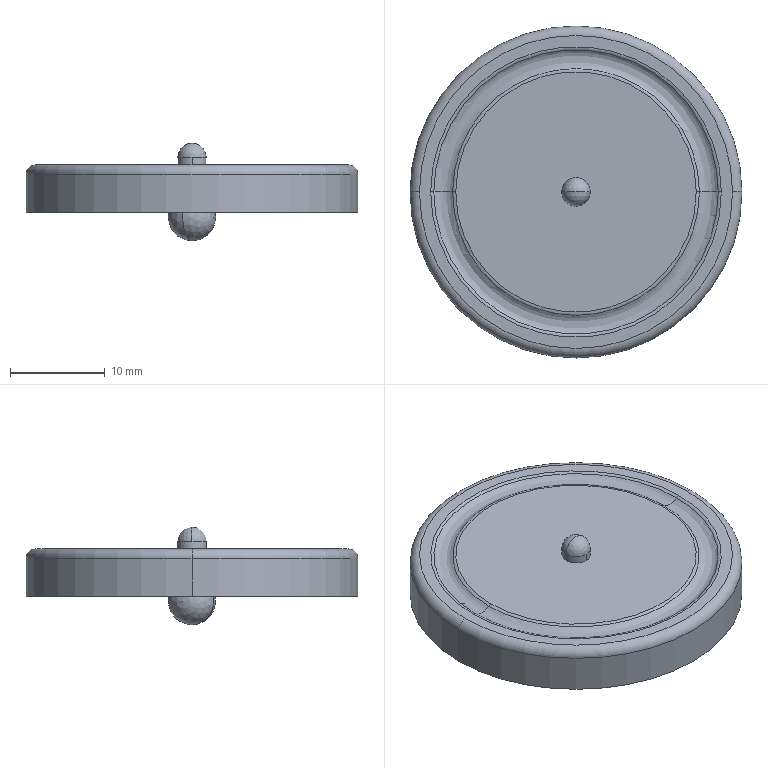Part | SolidWorks | features Fillet 2, RevCut 2, Revolution 2, Extrusion 1 | 2 solids | 24 faces | box 35 x 35 x 10.3 mm | volume 4614 mm3 | torus 10 | cylinder 6 | sphere 4 | plane 4 | commonest cylinder face diameters 3 x2 11 x2 35 x2
STEP:
#1=CARTESIAN_POINT('',(-121.531,115.619,-3.));
#2=VERTEX_POINT('',#1);
#3=CARTESIAN_POINT('',(-121.531,115.619,2.));
#4=VERTEX_POINT('',#3);
#5=CARTESIAN_POINT('',(-121.531,115.619,-0.5));
#6=DIRECTION('',(0.9209,-0.3898,0.));
#7=DIRECTION('',(0.3898,0.9209,0.));
#8=AXIS2_PLACEMENT_3D('',#5,#6,#7);
#9=CIRCLE('',#8,2.5);
#10=EDGE_CURVE('',#2,#4,#9,.T.);
#11=ORIENTED_EDGE('',*,*,#10,.F.);
#12=CARTESIAN_POINT('',(-121.531,115.619,-0.5));
#13=DIRECTION('',(-0.9209,0.3898,0.));
#14=DIRECTION('',(-0.3898,-0.9209,0.));
#15=AXIS2_PLACEMENT_3D('',#12,#13,#14);
#16=CIRCLE('',#15,2.5);
#17=EDGE_CURVE('',#2,#4,#16,.T.);
#18=ORIENTED_EDGE('',*,*,#17,.T.);
#19=EDGE_LOOP('',(#11,#18));
#20=FACE_OUTER_BOUND('',#19,.T.);
#21=CARTESIAN_POINT('',(-121.531,115.619,-0.5));
#22=DIRECTION('',(-0.9209,0.3898,0.));
#23=DIRECTION('',(0.3898,0.9209,0.));
#24=AXIS2_PLACEMENT_3D('',#21,#22,#23);
#25=SPHERICAL_SURFACE('',#24,2.5);
#26=ADVANCED_FACE('',(#20),#25,.T.);
#27=ORIENTED_EDGE('',*,*,#17,.F.);
#28=ORIENTED_EDGE('',*,*,#10,.T.);
#29=EDGE_LOOP('',(#27,#28));
#30=FACE_OUTER_BOUND('',#29,.T.);
#31=CARTESIAN_POINT('',(-121.531,115.619,-0.5));
#32=DIRECTION('',(-0.9209,0.3898,0.));
#33=DIRECTION('',(0.3898,0.9209,0.));
#34=AXIS2_PLACEMENT_3D('',#31,#32,#33);
#35=SPHERICAL_SURFACE('',#34,2.5);
#36=ADVANCED_FACE('',(#30),#35,.T.);
#37=CLOSED_SHELL('',(#26,#36));
#38=MANIFOLD_SOLID_BREP('',#37);
#39=CARTESIAN_POINT('',(-120.031,115.619,5.8));
#40=VERTEX_POINT('',#39);
#41=CARTESIAN_POINT('',(-121.531,114.119,5.8));
#42=VERTEX_POINT('',#41);
#43=CARTESIAN_POINT('',(-121.531,115.619,5.8));
#44=DIRECTION('',(0.,0.,-1.));
#45=DIRECTION('',(0.,1.,0.));
#46=AXIS2_PLACEMENT_3D('',#43,#44,#45);
#47=CIRCLE('',#46,1.5);
#48=EDGE_CURVE('',#40,#42,#47,.T.);
#49=ORIENTED_EDGE('',*,*,#48,.T.);
#50=CARTESIAN_POINT('',(-121.531,114.119,5.));
#51=VERTEX_POINT('',#50);
#52=CARTESIAN_POINT('',(-121.531,114.119,0.));
#53=DIRECTION('',(0.,0.,-1.));
#54=VECTOR('',#53,1000.);
#55=LINE('',#52,#54);
#56=EDGE_CURVE('',#42,#51,#55,.T.);
#57=ORIENTED_EDGE('',*,*,#56,.T.);
#58=CARTESIAN_POINT('',(-121.531,117.119,5.));
#59=VERTEX_POINT('',#58);
#60=CARTESIAN_POINT('',(-121.531,115.619,5.));
#61=DIRECTION('',(0.,0.,-1.));
#62=DIRECTION('',(1.,0.,0.));
#63=AXIS2_PLACEMENT_3D('',#60,#61,#62);
#64=CIRCLE('',#63,1.5);
#65=EDGE_CURVE('',#59,#51,#64,.T.);
#66=ORIENTED_EDGE('',*,*,#65,.F.);
#67=CARTESIAN_POINT('',(-121.531,117.119,5.8));
#68=VERTEX_POINT('',#67);
#69=CARTESIAN_POINT('',(-121.531,117.119,0.));
#70=DIRECTION('',(0.,0.,-1.));
#71=VECTOR('',#70,1000.);
#72=LINE('',#69,#71);
#73=EDGE_CURVE('',#68,#59,#72,.T.);
#74=ORIENTED_EDGE('',*,*,#73,.F.);
#75=CARTESIAN_POINT('',(-121.531,115.619,5.8));
#76=DIRECTION('',(0.,0.,-1.));
#77=DIRECTION('',(0.,1.,0.));
#78=AXIS2_PLACEMENT_3D('',#75,#76,#77);
#79=CIRCLE('',#78,1.5);
#80=EDGE_CURVE('',#68,#40,#79,.T.);
#81=ORIENTED_EDGE('',*,*,#80,.T.);
#82=EDGE_LOOP('',(#49,#57,#66,#74,#81));
#83=FACE_OUTER_BOUND('',#82,.T.);
#84=CARTESIAN_POINT('',(-121.531,115.619,0.));
#85=DIRECTION('',(0.,0.,-1.));
#86=DIRECTION('',(0.,1.,0.));
#87=AXIS2_PLACEMENT_3D('',#84,#85,#86);
#88=CYLINDRICAL_SURFACE('',#87,1.5);
#89=ADVANCED_FACE('',(#83),#88,.T.);
#90=CARTESIAN_POINT('',(-121.531,115.619,7.3));
#91=VERTEX_POINT('',#90);
#92=CARTESIAN_POINT('',(-121.531,115.619,5.8));
#93=DIRECTION('',(0.,1.,0.));
#94=DIRECTION('',(0.,0.,1.));
#95=AXIS2_PLACEMENT_3D('',#92,#93,#94);
#96=CIRCLE('',#95,1.5);
#97=EDGE_CURVE('',#91,#40,#96,.T.);
#98=ORIENTED_EDGE('',*,*,#97,.F.);
#99=CARTESIAN_POINT('',(-123.031,115.619,5.8));
#100=VERTEX_POINT('',#99);
#101=CARTESIAN_POINT('',(-121.531,115.619,5.8));
#102=DIRECTION('',(0.,-1.,0.));
#103=DIRECTION('',(0.,0.,-1.));
#104=AXIS2_PLACEMENT_3D('',#101,#102,#103);
#105=CIRCLE('',#104,1.5);
#106=EDGE_CURVE('',#91,#100,#105,.T.);
#107=ORIENTED_EDGE('',*,*,#106,.T.);
#108=CARTESIAN_POINT('',(-121.531,115.619,5.8));
#109=DIRECTION('',(0.,0.,-1.));
#110=DIRECTION('',(0.,1.,0.));
#111=AXIS2_PLACEMENT_3D('',#108,#109,#110);
#112=CIRCLE('',#111,1.5);
#113=EDGE_CURVE('',#42,#100,#112,.T.);
#114=ORIENTED_EDGE('',*,*,#113,.F.);
#115=ORIENTED_EDGE('',*,*,#48,.F.);
#116=EDGE_LOOP('',(#98,#107,#114,#115));
#117=FACE_OUTER_BOUND('',#116,.T.);
#118=CARTESIAN_POINT('',(-121.531,115.619,5.8));
#119=DIRECTION('',(0.,-1.,0.));
#120=DIRECTION('',(1.,0.,0.));
#121=AXIS2_PLACEMENT_3D('',#118,#119,#120);
#122=SPHERICAL_SURFACE('',#121,1.5);
#123=ADVANCED_FACE('',(#117),#122,.T.);
#124=CARTESIAN_POINT('',(-108.854,115.619,5.));
#125=VERTEX_POINT('',#124);
#126=CARTESIAN_POINT('',(-134.208,115.619,5.));
#127=VERTEX_POINT('',#126);
#128=CARTESIAN_POINT('',(-121.531,115.619,5.));
#129=DIRECTION('',(0.,0.,1.));
#130=DIRECTION('',(1.,0.,0.));
#131=AXIS2_PLACEMENT_3D('',#128,#129,#130);
#132=CIRCLE('',#131,12.677);
#133=EDGE_CURVE('',#125,#127,#132,.T.);
#134=ORIENTED_EDGE('',*,*,#133,.F.);
#135=CARTESIAN_POINT('',(-108.523,115.619,4.875));
#136=VERTEX_POINT('',#135);
#137=CARTESIAN_POINT('',(-108.854,115.619,4.5));
#138=DIRECTION('',(0.,1.,0.));
#139=DIRECTION('',(-1.,0.,0.));
#140=AXIS2_PLACEMENT_3D('',#137,#138,#139);
#141=CIRCLE('',#140,0.5);
#142=EDGE_CURVE('',#125,#136,#141,.T.);
#143=ORIENTED_EDGE('',*,*,#142,.T.);
#144=CARTESIAN_POINT('',(-134.539,115.619,4.875));
#145=VERTEX_POINT('',#144);
#146=CARTESIAN_POINT('',(-121.531,115.619,4.875));
#147=DIRECTION('',(0.,0.,-1.));
#148=DIRECTION('',(1.,0.,0.));
#149=AXIS2_PLACEMENT_3D('',#146,#147,#148);
#150=CIRCLE('',#149,13.008);
#151=EDGE_CURVE('',#145,#136,#150,.T.);
#152=ORIENTED_EDGE('',*,*,#151,.F.);
#153=CARTESIAN_POINT('',(-134.208,115.619,4.5));
#154=DIRECTION('',(0.,-1.,0.));
#155=DIRECTION('',(0.,0.,-1.));
#156=AXIS2_PLACEMENT_3D('',#153,#154,#155);
#157=CIRCLE('',#156,0.5);
#158=EDGE_CURVE('',#127,#145,#157,.T.);
#159=ORIENTED_EDGE('',*,*,#158,.F.);
#160=EDGE_LOOP('',(#134,#143,#152,#159));
#161=FACE_OUTER_BOUND('',#160,.T.);
#162=CARTESIAN_POINT('',(-121.531,115.619,4.5));
#163=DIRECTION('',(0.,0.,-1.));
#164=DIRECTION('',(-1.,0.,0.));
#165=AXIS2_PLACEMENT_3D('',#162,#163,#164);
#166=TOROIDAL_SURFACE('',#165,12.677,0.5);
#167=ADVANCED_FACE('',(#161),#166,.T.);
#168=CARTESIAN_POINT('',(-136.854,115.619,5.));
#169=VERTEX_POINT('',#168);
#170=CARTESIAN_POINT('',(-106.208,115.619,5.));
#171=VERTEX_POINT('',#170);
#172=CARTESIAN_POINT('',(-121.531,115.619,5.));
#173=DIRECTION('',(0.,0.,-1.));
#174=DIRECTION('',(1.,0.,0.));
#175=AXIS2_PLACEMENT_3D('',#172,#173,#174);
#176=CIRCLE('',#175,15.323);
#177=EDGE_CURVE('',#169,#171,#176,.T.);
#178=ORIENTED_EDGE('',*,*,#177,.F.);
#179=CARTESIAN_POINT('',(-136.523,115.619,4.875));
#180=VERTEX_POINT('',#179);
#181=CARTESIAN_POINT('',(-136.854,115.619,4.5));
#182=DIRECTION('',(0.,1.,0.));
#183=DIRECTION('',(-1.,0.,0.));
#184=AXIS2_PLACEMENT_3D('',#181,#182,#183);
#185=CIRCLE('',#184,0.5);
#186=EDGE_CURVE('',#169,#180,#185,.T.);
#187=ORIENTED_EDGE('',*,*,#186,.T.);
#188=CARTESIAN_POINT('',(-106.539,115.619,4.875));
#189=VERTEX_POINT('',#188);
#190=CARTESIAN_POINT('',(-121.531,115.619,4.875));
#191=DIRECTION('',(0.,0.,1.));
#192=DIRECTION('',(1.,0.,0.));
#193=AXIS2_PLACEMENT_3D('',#190,#191,#192);
#194=CIRCLE('',#193,14.992);
#195=EDGE_CURVE('',#189,#180,#194,.T.);
#196=ORIENTED_EDGE('',*,*,#195,.F.);
#197=CARTESIAN_POINT('',(-106.208,115.619,4.5));
#198=DIRECTION('',(0.,-1.,0.));
#199=DIRECTION('',(0.,0.,-1.));
#200=AXIS2_PLACEMENT_3D('',#197,#198,#199);
#201=CIRCLE('',#200,0.5);
#202=EDGE_CURVE('',#171,#189,#201,.T.);
#203=ORIENTED_EDGE('',*,*,#202,.F.);
#204=EDGE_LOOP('',(#178,#187,#196,#203));
#205=FACE_OUTER_BOUND('',#204,.T.);
#206=CARTESIAN_POINT('',(-121.531,115.619,4.5));
#207=DIRECTION('',(0.,0.,1.));
#208=DIRECTION('',(1.,0.,0.));
#209=AXIS2_PLACEMENT_3D('',#206,#207,#208);
#210=TOROIDAL_SURFACE('',#209,15.323,0.5);
#211=ADVANCED_FACE('',(#205),#210,.T.);
#212=CARTESIAN_POINT('',(-139.031,115.619,4.));
#213=VERTEX_POINT('',#212);
#214=CARTESIAN_POINT('',(-104.031,115.619,4.));
#215=VERTEX_POINT('',#214);
#216=CARTESIAN_POINT('',(-121.531,115.619,4.));
#217=DIRECTION('',(0.,0.,-1.));
#218=DIRECTION('',(1.,0.,0.));
#219=AXIS2_PLACEMENT_3D('',#216,#217,#218);
#220=CIRCLE('',#219,17.5);
#221=EDGE_CURVE('',#213,#215,#220,.T.);
#222=ORIENTED_EDGE('',*,*,#221,.F.);
#223=CARTESIAN_POINT('',(-138.031,115.619,5.));
#224=VERTEX_POINT('',#223);
#225=CARTESIAN_POINT('',(-138.031,115.619,4.));
#226=DIRECTION('',(0.,1.,0.));
#227=DIRECTION('',(-1.,0.,0.));
#228=AXIS2_PLACEMENT_3D('',#225,#226,#227);
#229=CIRCLE('',#228,1.);
#230=EDGE_CURVE('',#213,#224,#229,.T.);
#231=ORIENTED_EDGE('',*,*,#230,.T.);
#232=CARTESIAN_POINT('',(-105.031,115.619,5.));
#233=VERTEX_POINT('',#232);
#234=CARTESIAN_POINT('',(-121.531,115.619,5.));
#235=DIRECTION('',(0.,0.,1.));
#236=DIRECTION('',(1.,0.,0.));
#237=AXIS2_PLACEMENT_3D('',#234,#235,#236);
#238=CIRCLE('',#237,16.5);
#239=EDGE_CURVE('',#233,#224,#238,.T.);
#240=ORIENTED_EDGE('',*,*,#239,.F.);
#241=CARTESIAN_POINT('',(-105.031,115.619,4.));
#242=DIRECTION('',(0.,-1.,0.));
#243=DIRECTION('',(0.,0.,-1.));
#244=AXIS2_PLACEMENT_3D('',#241,#242,#243);
#245=CIRCLE('',#244,1.);
#246=EDGE_CURVE('',#215,#233,#245,.T.);
#247=ORIENTED_EDGE('',*,*,#246,.F.);
#248=EDGE_LOOP('',(#222,#231,#240,#247));
#249=FACE_OUTER_BOUND('',#248,.T.);
#250=CARTESIAN_POINT('',(-121.531,115.619,4.));
#251=DIRECTION('',(0.,0.,1.));
#252=DIRECTION('',(1.,0.,0.));
#253=AXIS2_PLACEMENT_3D('',#250,#251,#252);
#254=TOROIDAL_SURFACE('',#253,16.5,1.);
#255=ADVANCED_FACE('',(#249),#254,.T.);
#256=CARTESIAN_POINT('',(-121.531,115.619,4.875));
#257=DIRECTION('',(0.,0.,-1.));
#258=DIRECTION('',(1.,0.,0.));
#259=AXIS2_PLACEMENT_3D('',#256,#257,#258);
#260=CIRCLE('',#259,13.008);
#261=EDGE_CURVE('',#136,#145,#260,.T.);
#262=ORIENTED_EDGE('',*,*,#261,.T.);
#263=CARTESIAN_POINT('',(-135.531,115.619,6.));
#264=DIRECTION('',(0.,1.,0.));
#265=DIRECTION('',(-1.,0.,0.));
#266=AXIS2_PLACEMENT_3D('',#263,#264,#265);
#267=CIRCLE('',#266,1.5);
#268=EDGE_CURVE('',#145,#180,#267,.T.);
#269=ORIENTED_EDGE('',*,*,#268,.T.);
#270=CARTESIAN_POINT('',(-121.531,115.619,4.875));
#271=DIRECTION('',(0.,0.,1.));
#272=DIRECTION('',(1.,0.,0.));
#273=AXIS2_PLACEMENT_3D('',#270,#271,#272);
#274=CIRCLE('',#273,14.992);
#275=EDGE_CURVE('',#180,#189,#274,.T.);
#276=ORIENTED_EDGE('',*,*,#275,.T.);
#277=CARTESIAN_POINT('',(-107.531,115.619,6.));
#278=DIRECTION('',(0.,-1.,0.));
#279=DIRECTION('',(0.,0.,-1.));
#280=AXIS2_PLACEMENT_3D('',#277,#278,#279);
#281=CIRCLE('',#280,1.5);
#282=EDGE_CURVE('',#136,#189,#281,.T.);
#283=ORIENTED_EDGE('',*,*,#282,.F.);
#284=EDGE_LOOP('',(#262,#269,#276,#283));
#285=FACE_OUTER_BOUND('',#284,.T.);
#286=CARTESIAN_POINT('',(-121.531,115.619,6.));
#287=DIRECTION('',(0.,0.,1.));
#288=DIRECTION('',(1.,0.,0.));
#289=AXIS2_PLACEMENT_3D('',#286,#287,#288);
#290=TOROIDAL_SURFACE('',#289,14.,1.5);
#291=ADVANCED_FACE('',(#285),#290,.F.);
#292=CARTESIAN_POINT('',(-121.531,121.119,0.));
#293=VERTEX_POINT('',#292);
#294=CARTESIAN_POINT('',(-121.531,110.119,0.));
#295=VERTEX_POINT('',#294);
#296=CARTESIAN_POINT('',(-121.531,115.619,0.));
#297=DIRECTION('',(0.,0.,1.));
#298=DIRECTION('',(0.,-1.,0.));
#299=AXIS2_PLACEMENT_3D('',#296,#297,#298);
#300=CIRCLE('',#299,5.5);
#301=EDGE_CURVE('',#293,#295,#300,.T.);
#302=ORIENTED_EDGE('',*,*,#301,.F.);
#303=CARTESIAN_POINT('',(-121.531,121.119,1.));
#304=VERTEX_POINT('',#303);
#305=CARTESIAN_POINT('',(-121.531,121.119,5.877));
#306=DIRECTION('',(0.,0.,1.));
#307=VECTOR('',#306,1000.);
#308=LINE('',#305,#307);
#309=EDGE_CURVE('',#293,#304,#308,.T.);
#310=ORIENTED_EDGE('',*,*,#309,.T.);
#311=CARTESIAN_POINT('',(-121.531,110.119,1.));
#312=VERTEX_POINT('',#311);
#313=CARTESIAN_POINT('',(-121.531,115.619,1.));
#314=DIRECTION('',(0.,0.,1.));
#315=DIRECTION('',(0.,-1.,0.));
#316=AXIS2_PLACEMENT_3D('',#313,#314,#315);
#317=CIRCLE('',#316,5.5);
#318=EDGE_CURVE('',#304,#312,#317,.T.);
#319=ORIENTED_EDGE('',*,*,#318,.T.);
#320=CARTESIAN_POINT('',(-121.531,110.119,5.877));
#321=DIRECTION('',(0.,0.,1.));
#322=VECTOR('',#321,1000.);
#323=LINE('',#320,#322);
#324=EDGE_CURVE('',#295,#312,#323,.T.);
#325=ORIENTED_EDGE('',*,*,#324,.F.);
#326=EDGE_LOOP('',(#302,#310,#319,#325));
#327=FACE_OUTER_BOUND('',#326,.T.);
#328=CARTESIAN_POINT('',(-121.531,115.619,5.877));
#329=DIRECTION('',(0.,0.,1.));
#330=DIRECTION('',(0.,-1.,0.));
#331=AXIS2_PLACEMENT_3D('',#328,#329,#330);
#332=CYLINDRICAL_SURFACE('',#331,5.5);
#333=ADVANCED_FACE('',(#327),#332,.F.);
#334=ORIENTED_EDGE('',*,*,#318,.F.);
#335=CARTESIAN_POINT('',(-121.531,120.119,2.));
#336=VERTEX_POINT('',#335);
#337=CARTESIAN_POINT('',(-121.531,120.119,1.));
#338=DIRECTION('',(1.,0.,0.));
#339=DIRECTION('',(0.,1.,0.));
#340=AXIS2_PLACEMENT_3D('',#337,#338,#339);
#341=CIRCLE('',#340,1.);
#342=EDGE_CURVE('',#304,#336,#341,.T.);
#343=ORIENTED_EDGE('',*,*,#342,.T.);
#344=CARTESIAN_POINT('',(-121.531,111.119,2.));
#345=VERTEX_POINT('',#344);
#346=CARTESIAN_POINT('',(-121.531,115.619,2.));
#347=DIRECTION('',(0.,0.,1.));
#348=DIRECTION('',(0.,-1.,0.));
#349=AXIS2_PLACEMENT_3D('',#346,#347,#348);
#350=CIRCLE('',#349,4.5);
#351=EDGE_CURVE('',#336,#345,#350,.T.);
#352=ORIENTED_EDGE('',*,*,#351,.T.);
#353=CARTESIAN_POINT('',(-121.531,111.119,1.));
#354=DIRECTION('',(-1.,0.,0.));
#355=DIRECTION('',(0.,0.,1.));
#356=AXIS2_PLACEMENT_3D('',#353,#354,#355);
#357=CIRCLE('',#356,1.);
#358=EDGE_CURVE('',#312,#345,#357,.T.);
#359=ORIENTED_EDGE('',*,*,#358,.F.);
#360=EDGE_LOOP('',(#334,#343,#352,#359));
#361=FACE_OUTER_BOUND('',#360,.T.);
#362=CARTESIAN_POINT('',(-121.531,115.619,1.));
#363=DIRECTION('',(0.,0.,1.));
#364=DIRECTION('',(0.,-1.,0.));
#365=AXIS2_PLACEMENT_3D('',#362,#363,#364);
#366=TOROIDAL_SURFACE('',#365,4.5,1.);
#367=ADVANCED_FACE('',(#361),#366,.F.);
#368=ORIENTED_EDGE('',*,*,#221,.T.);
#369=CARTESIAN_POINT('',(-104.031,115.619,0.));
#370=VERTEX_POINT('',#369);
#371=CARTESIAN_POINT('',(-104.031,115.619,5.));
#372=DIRECTION('',(0.,0.,-1.));
#373=VECTOR('',#372,1000.);
#374=LINE('',#371,#373);
#375=EDGE_CURVE('',#215,#370,#374,.T.);
#376=ORIENTED_EDGE('',*,*,#375,.T.);
#377=CARTESIAN_POINT('',(-139.031,115.619,0.));
#378=VERTEX_POINT('',#377);
#379=CARTESIAN_POINT('',(-121.531,115.619,0.));
#380=DIRECTION('',(0.,0.,1.));
#381=DIRECTION('',(1.,0.,0.));
#382=AXIS2_PLACEMENT_3D('',#379,#380,#381);
#383=CIRCLE('',#382,17.5);
#384=EDGE_CURVE('',#370,#378,#383,.T.);
#385=ORIENTED_EDGE('',*,*,#384,.T.);
#386=CARTESIAN_POINT('',(-139.031,115.619,5.));
#387=DIRECTION('',(0.,0.,-1.));
#388=VECTOR('',#387,1000.);
#389=LINE('',#386,#388);
#390=EDGE_CURVE('',#213,#378,#389,.T.);
#391=ORIENTED_EDGE('',*,*,#390,.F.);
#392=EDGE_LOOP('',(#368,#376,#385,#391));
#393=FACE_OUTER_BOUND('',#392,.T.);
#394=CARTESIAN_POINT('',(-121.531,115.619,5.));
#395=DIRECTION('',(0.,0.,-1.));
#396=DIRECTION('',(-1.,0.,0.));
#397=AXIS2_PLACEMENT_3D('',#394,#395,#396);
#398=CYLINDRICAL_SURFACE('',#397,17.5);
#399=ADVANCED_FACE('',(#393),#398,.T.);
#400=CARTESIAN_POINT('',(-121.531,115.619,5.));
#401=DIRECTION('',(0.,0.,-1.));
#402=DIRECTION('',(1.,0.,0.));
#403=AXIS2_PLACEMENT_3D('',#400,#401,#402);
#404=CIRCLE('',#403,15.323);
#405=EDGE_CURVE('',#171,#169,#404,.T.);
#406=ORIENTED_EDGE('',*,*,#405,.T.);
#407=ORIENTED_EDGE('',*,*,#177,.T.);
#408=EDGE_LOOP('',(#406,#407));
#409=FACE_BOUND('',#408,.T.);
#410=ORIENTED_EDGE('',*,*,#239,.T.);
#411=CARTESIAN_POINT('',(-121.531,115.619,5.));
#412=DIRECTION('',(0.,0.,1.));
#413=DIRECTION('',(1.,0.,0.));
#414=AXIS2_PLACEMENT_3D('',#411,#412,#413);
#415=CIRCLE('',#414,16.5);
#416=EDGE_CURVE('',#224,#233,#415,.T.);
#417=ORIENTED_EDGE('',*,*,#416,.T.);
#418=EDGE_LOOP('',(#410,#417));
#419=FACE_OUTER_BOUND('',#418,.T.);
#420=CARTESIAN_POINT('',(-121.531,115.619,5.));
#421=DIRECTION('',(0.,0.,1.));
#422=DIRECTION('',(1.,0.,0.));
#423=AXIS2_PLACEMENT_3D('',#420,#421,#422);
#424=PLANE('',#423);
#425=ADVANCED_FACE('',(#409,#419),#424,.T.);
#426=ORIENTED_EDGE('',*,*,#375,.F.);
#427=CARTESIAN_POINT('',(-121.531,115.619,4.));
#428=DIRECTION('',(0.,0.,-1.));
#429=DIRECTION('',(1.,0.,0.));
#430=AXIS2_PLACEMENT_3D('',#427,#428,#429);
#431=CIRCLE('',#430,17.5);
#432=EDGE_CURVE('',#215,#213,#431,.T.);
#433=ORIENTED_EDGE('',*,*,#432,.T.);
#434=ORIENTED_EDGE('',*,*,#390,.T.);
#435=CARTESIAN_POINT('',(-121.531,115.619,0.));
#436=DIRECTION('',(0.,0.,1.));
#437=DIRECTION('',(1.,0.,0.));
#438=AXIS2_PLACEMENT_3D('',#435,#436,#437);
#439=CIRCLE('',#438,17.5);
#440=EDGE_CURVE('',#378,#370,#439,.T.);
#441=ORIENTED_EDGE('',*,*,#440,.T.);
#442=EDGE_LOOP('',(#426,#433,#434,#441));
#443=FACE_OUTER_BOUND('',#442,.T.);
#444=CARTESIAN_POINT('',(-121.531,115.619,5.));
#445=DIRECTION('',(0.,0.,-1.));
#446=DIRECTION('',(-1.,0.,0.));
#447=AXIS2_PLACEMENT_3D('',#444,#445,#446);
#448=CYLINDRICAL_SURFACE('',#447,17.5);
#449=ADVANCED_FACE('',(#443),#448,.T.);
#450=CARTESIAN_POINT('',(-121.531,115.619,0.));
#451=DIRECTION('',(0.,0.,1.));
#452=DIRECTION('',(0.,-1.,0.));
#453=AXIS2_PLACEMENT_3D('',#450,#451,#452);
#454=CIRCLE('',#453,5.5);
#455=EDGE_CURVE('',#295,#293,#454,.T.);
#456=ORIENTED_EDGE('',*,*,#455,.T.);
#457=ORIENTED_EDGE('',*,*,#301,.T.);
#458=EDGE_LOOP('',(#456,#457));
#459=FACE_BOUND('',#458,.T.);
#460=ORIENTED_EDGE('',*,*,#440,.F.);
#461=ORIENTED_EDGE('',*,*,#384,.F.);
#462=EDGE_LOOP('',(#460,#461));
#463=FACE_OUTER_BOUND('',#462,.T.);
#464=CARTESIAN_POINT('',(-121.531,115.619,0.));
#465=DIRECTION('',(0.,0.,1.));
#466=DIRECTION('',(1.,0.,0.));
#467=AXIS2_PLACEMENT_3D('',#464,#465,#466);
#468=PLANE('',#467);
#469=ADVANCED_FACE('',(#459,#463),#468,.F.);
#470=CARTESIAN_POINT('',(-121.531,115.619,2.));
#471=DIRECTION('',(0.,0.,1.));
#472=DIRECTION('',(0.,-1.,0.));
#473=AXIS2_PLACEMENT_3D('',#470,#471,#472);
#474=CIRCLE('',#473,4.5);
#475=EDGE_CURVE('',#345,#336,#474,.T.);
#476=ORIENTED_EDGE('',*,*,#475,.F.);
#477=ORIENTED_EDGE('',*,*,#351,.F.);
#478=EDGE_LOOP('',(#476,#477));
#479=FACE_OUTER_BOUND('',#478,.T.);
#480=CARTESIAN_POINT('',(-121.531,115.619,2.));
#481=DIRECTION('',(0.,0.,1.));
#482=DIRECTION('',(0.,-1.,0.));
#483=AXIS2_PLACEMENT_3D('',#480,#481,#482);
#484=PLANE('',#483);
#485=ADVANCED_FACE('',(#479),#484,.F.);
#486=ORIENTED_EDGE('',*,*,#342,.F.);
#487=CARTESIAN_POINT('',(-121.531,115.619,1.));
#488=DIRECTION('',(0.,0.,1.));
#489=DIRECTION('',(0.,-1.,0.));
#490=AXIS2_PLACEMENT_3D('',#487,#488,#489);
#491=CIRCLE('',#490,5.5);
#492=EDGE_CURVE('',#312,#304,#491,.T.);
#493=ORIENTED_EDGE('',*,*,#492,.F.);
#494=ORIENTED_EDGE('',*,*,#358,.T.);
#495=ORIENTED_EDGE('',*,*,#475,.T.);
#496=EDGE_LOOP('',(#486,#493,#494,#495));
#497=FACE_OUTER_BOUND('',#496,.T.);
#498=CARTESIAN_POINT('',(-121.531,115.619,1.));
#499=DIRECTION('',(0.,0.,1.));
#500=DIRECTION('',(0.,-1.,0.));
#501=AXIS2_PLACEMENT_3D('',#498,#499,#500);
#502=TOROIDAL_SURFACE('',#501,4.5,1.);
#503=ADVANCED_FACE('',(#497),#502,.F.);
#504=ORIENTED_EDGE('',*,*,#309,.F.);
#505=ORIENTED_EDGE('',*,*,#455,.F.);
#506=ORIENTED_EDGE('',*,*,#324,.T.);
#507=ORIENTED_EDGE('',*,*,#492,.T.);
#508=EDGE_LOOP('',(#504,#505,#506,#507));
#509=FACE_OUTER_BOUND('',#508,.T.);
#510=CARTESIAN_POINT('',(-121.531,115.619,5.877));
#511=DIRECTION('',(0.,0.,1.));
#512=DIRECTION('',(0.,-1.,0.));
#513=AXIS2_PLACEMENT_3D('',#510,#511,#512);
#514=CYLINDRICAL_SURFACE('',#513,5.5);
#515=ADVANCED_FACE('',(#509),#514,.F.);
#516=ORIENTED_EDGE('',*,*,#268,.F.);
#517=ORIENTED_EDGE('',*,*,#151,.T.);
#518=ORIENTED_EDGE('',*,*,#282,.T.);
#519=ORIENTED_EDGE('',*,*,#195,.T.);
#520=EDGE_LOOP('',(#516,#517,#518,#519));
#521=FACE_OUTER_BOUND('',#520,.T.);
#522=CARTESIAN_POINT('',(-121.531,115.619,6.));
#523=DIRECTION('',(0.,0.,1.));
#524=DIRECTION('',(1.,0.,0.));
#525=AXIS2_PLACEMENT_3D('',#522,#523,#524);
#526=TOROIDAL_SURFACE('',#525,14.,1.5);
#527=ADVANCED_FACE('',(#521),#526,.F.);
#528=ORIENTED_EDGE('',*,*,#65,.T.);
#529=CARTESIAN_POINT('',(-121.531,115.619,5.));
#530=DIRECTION('',(0.,0.,-1.));
#531=DIRECTION('',(1.,0.,0.));
#532=AXIS2_PLACEMENT_3D('',#529,#530,#531);
#533=CIRCLE('',#532,1.5);
#534=EDGE_CURVE('',#51,#59,#533,.T.);
#535=ORIENTED_EDGE('',*,*,#534,.T.);
#536=EDGE_LOOP('',(#528,#535));
#537=FACE_BOUND('',#536,.T.);
#538=CARTESIAN_POINT('',(-121.531,115.619,5.));
#539=DIRECTION('',(0.,0.,1.));
#540=DIRECTION('',(1.,0.,0.));
#541=AXIS2_PLACEMENT_3D('',#538,#539,#540);
#542=CIRCLE('',#541,12.677);
#543=EDGE_CURVE('',#127,#125,#542,.T.);
#544=ORIENTED_EDGE('',*,*,#543,.T.);
#545=ORIENTED_EDGE('',*,*,#133,.T.);
#546=EDGE_LOOP('',(#544,#545));
#547=FACE_OUTER_BOUND('',#546,.T.);
#548=CARTESIAN_POINT('',(-121.531,115.619,5.));
#549=DIRECTION('',(0.,0.,1.));
#550=DIRECTION('',(1.,0.,0.));
#551=AXIS2_PLACEMENT_3D('',#548,#549,#550);
#552=PLANE('',#551);
#553=ADVANCED_FACE('',(#537,#547),#552,.T.);
#554=ORIENTED_EDGE('',*,*,#230,.F.);
#555=ORIENTED_EDGE('',*,*,#432,.F.);
#556=ORIENTED_EDGE('',*,*,#246,.T.);
#557=ORIENTED_EDGE('',*,*,#416,.F.);
#558=EDGE_LOOP('',(#554,#555,#556,#557));
#559=FACE_OUTER_BOUND('',#558,.T.);
#560=CARTESIAN_POINT('',(-121.531,115.619,4.));
#561=DIRECTION('',(0.,0.,1.));
#562=DIRECTION('',(1.,0.,0.));
#563=AXIS2_PLACEMENT_3D('',#560,#561,#562);
#564=TOROIDAL_SURFACE('',#563,16.5,1.);
#565=ADVANCED_FACE('',(#559),#564,.T.);
#566=ORIENTED_EDGE('',*,*,#186,.F.);
#567=ORIENTED_EDGE('',*,*,#405,.F.);
#568=ORIENTED_EDGE('',*,*,#202,.T.);
#569=ORIENTED_EDGE('',*,*,#275,.F.);
#570=EDGE_LOOP('',(#566,#567,#568,#569));
#571=FACE_OUTER_BOUND('',#570,.T.);
#572=CARTESIAN_POINT('',(-121.531,115.619,4.5));
#573=DIRECTION('',(0.,0.,1.));
#574=DIRECTION('',(1.,0.,0.));
#575=AXIS2_PLACEMENT_3D('',#572,#573,#574);
#576=TOROIDAL_SURFACE('',#575,15.323,0.5);
#577=ADVANCED_FACE('',(#571),#576,.T.);
#578=ORIENTED_EDGE('',*,*,#142,.F.);
#579=ORIENTED_EDGE('',*,*,#543,.F.);
#580=ORIENTED_EDGE('',*,*,#158,.T.);
#581=ORIENTED_EDGE('',*,*,#261,.F.);
#582=EDGE_LOOP('',(#578,#579,#580,#581));
#583=FACE_OUTER_BOUND('',#582,.T.);
#584=CARTESIAN_POINT('',(-121.531,115.619,4.5));
#585=DIRECTION('',(0.,0.,-1.));
#586=DIRECTION('',(-1.,0.,0.));
#587=AXIS2_PLACEMENT_3D('',#584,#585,#586);
#588=TOROIDAL_SURFACE('',#587,12.677,0.5);
#589=ADVANCED_FACE('',(#583),#588,.T.);
#590=ORIENTED_EDGE('',*,*,#106,.F.);
#591=ORIENTED_EDGE('',*,*,#97,.T.);
#592=ORIENTED_EDGE('',*,*,#80,.F.);
#593=CARTESIAN_POINT('',(-121.531,115.619,5.8));
#594=DIRECTION('',(0.,0.,-1.));
#595=DIRECTION('',(0.,1.,0.));
#596=AXIS2_PLACEMENT_3D('',#593,#594,#595);
#597=CIRCLE('',#596,1.5);
#598=EDGE_CURVE('',#100,#68,#597,.T.);
#599=ORIENTED_EDGE('',*,*,#598,.F.);
#600=EDGE_LOOP('',(#590,#591,#592,#599));
#601=FACE_OUTER_BOUND('',#600,.T.);
#602=CARTESIAN_POINT('',(-121.531,115.619,5.8));
#603=DIRECTION('',(0.,-1.,0.));
#604=DIRECTION('',(1.,0.,0.));
#605=AXIS2_PLACEMENT_3D('',#602,#603,#604);
#606=SPHERICAL_SURFACE('',#605,1.5);
#607=ADVANCED_FACE('',(#601),#606,.T.);
#608=ORIENTED_EDGE('',*,*,#56,.F.);
#609=ORIENTED_EDGE('',*,*,#113,.T.);
#610=ORIENTED_EDGE('',*,*,#598,.T.);
#611=ORIENTED_EDGE('',*,*,#73,.T.);
#612=ORIENTED_EDGE('',*,*,#534,.F.);
#613=EDGE_LOOP('',(#608,#609,#610,#611,#612));
#614=FACE_OUTER_BOUND('',#613,.T.);
#615=CARTESIAN_POINT('',(-121.531,115.619,0.));
#616=DIRECTION('',(0.,0.,-1.));
#617=DIRECTION('',(0.,1.,0.));
#618=AXIS2_PLACEMENT_3D('',#615,#616,#617);
#619=CYLINDRICAL_SURFACE('',#618,1.5);
#620=ADVANCED_FACE('',(#614),#619,.T.);
#621=CLOSED_SHELL('',(#89,#123,#167,#211,#255,#291,#333,#367,#399,#425,#449,#469,#485,#503,#515,#527,#553,#565,#577,#589,#607,#620));
#622=MANIFOLD_SOLID_BREP('',#621);
#623=CARTESIAN_POINT('',(0.,0.,0.));
#624=DIRECTION('',(0.,0.,1.));
#625=DIRECTION('',(1.,0.,0.));
#626=AXIS2_PLACEMENT_3D('',#623,#624,#625);
#627=(LENGTH_UNIT()NAMED_UNIT(*)SI_UNIT(.MILLI.,.METRE.));
#628=UNCERTAINTY_MEASURE_WITH_UNIT(LENGTH_MEASURE(0.00001),#627,'','');
#629=(NAMED_UNIT(*)PLANE_ANGLE_UNIT()SI_UNIT($,.RADIAN.));
#630=(NAMED_UNIT(*)SI_UNIT($,.STERADIAN.)SOLID_ANGLE_UNIT());
#631=(GEOMETRIC_REPRESENTATION_CONTEXT(3)GLOBAL_UNCERTAINTY_ASSIGNED_CONTEXT((#628))GLOBAL_UNIT_ASSIGNED_CONTEXT((#627,#629,#630))REPRESENTATION_CONTEXT('',''));
#632=ADVANCED_BREP_SHAPE_REPRESENTATION('',(#38,#622,#626),#631);